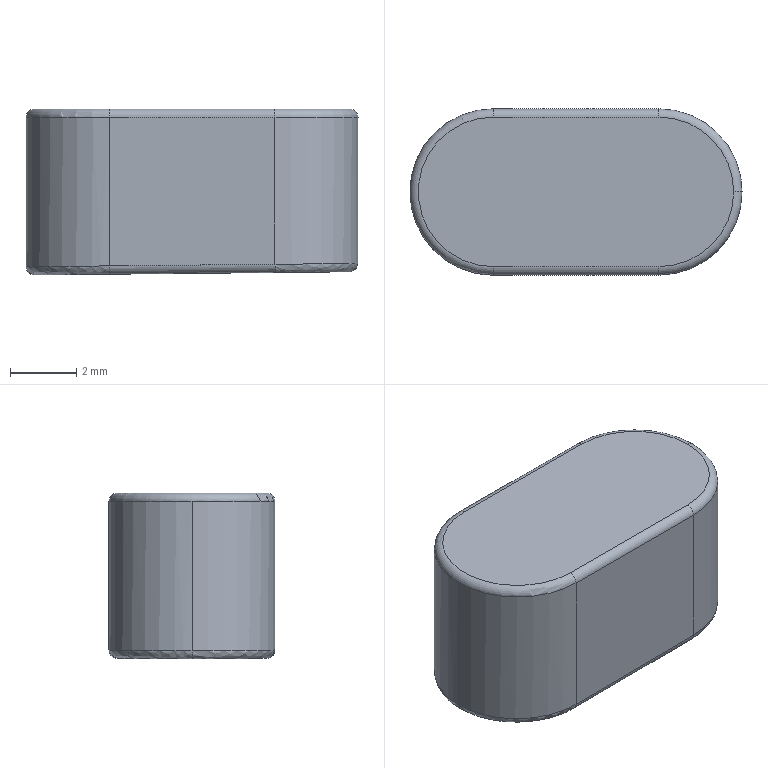Part | SolidWorks | features Cut 1, Extrusion 1, Fillet 1 | 1 solid | 17 faces | box 10 x 5 x 4.997 mm | volume 220.26 mm3 | cylinder 7 | plane 4 | spline 3 | torus 3 | commonest cylinder face diameters 0.5 x4 5 x3
STEP:
#1=CARTESIAN_POINT('',(-4.748,0.,0.002525));
#2=VERTEX_POINT('',#1);
#3=CARTESIAN_POINT('',(-2.498,2.25,0.02502));
#4=VERTEX_POINT('',#3);
#5=CARTESIAN_POINT('',(-4.748,0.,0.002525));
#6=CARTESIAN_POINT('',(-4.748,1.318,0.002525));
#7=CARTESIAN_POINT('',(-3.816,2.25,0.01184));
#8=CARTESIAN_POINT('',(-2.498,2.25,0.02502));
#9=(BOUNDED_CURVE()B_SPLINE_CURVE(3,(#5,#6,#7,#8),.UNSPECIFIED.,.F.,.F.)B_SPLINE_CURVE_WITH_KNOTS((4,4),(0.,1.571),.UNSPECIFIED.)CURVE()GEOMETRIC_REPRESENTATION_ITEM()RATIONAL_B_SPLINE_CURVE((1.,0.8047,0.8047,1.))REPRESENTATION_ITEM(''));
#10=EDGE_CURVE('',#2,#4,#9,.T.);
#11=ORIENTED_EDGE('',*,*,#10,.F.);
#12=CARTESIAN_POINT('',(-5.,0.,0.2525));
#13=VERTEX_POINT('',#12);
#14=CARTESIAN_POINT('',(-4.75,0.,0.2525));
#15=DIRECTION('',(0.,1.,0.));
#16=DIRECTION('',(0.,0.,1.));
#17=AXIS2_PLACEMENT_3D('',#14,#15,#16);
#18=CIRCLE('',#17,0.25);
#19=EDGE_CURVE('',#2,#13,#18,.T.);
#20=ORIENTED_EDGE('',*,*,#19,.T.);
#21=CARTESIAN_POINT('',(-2.5,2.5,0.275));
#22=VERTEX_POINT('',#21);
#23=CARTESIAN_POINT('',(-2.5,2.5,0.275));
#24=CARTESIAN_POINT('',(-3.964,2.5,0.2618));
#25=CARTESIAN_POINT('',(-5.,1.464,0.2525));
#26=CARTESIAN_POINT('',(-5.,0.,0.2525));
#27=(BOUNDED_CURVE()B_SPLINE_CURVE(3,(#23,#24,#25,#26),.UNSPECIFIED.,.F.,.F.)B_SPLINE_CURVE_WITH_KNOTS((4,4),(4.712,6.283),.UNSPECIFIED.)CURVE()GEOMETRIC_REPRESENTATION_ITEM()RATIONAL_B_SPLINE_CURVE((1.,0.8047,0.8047,1.))REPRESENTATION_ITEM(''));
#28=EDGE_CURVE('',#22,#13,#27,.T.);
#29=ORIENTED_EDGE('',*,*,#28,.F.);
#30=CARTESIAN_POINT('',(-2.5,2.25,0.275));
#31=DIRECTION('',(-1.,0.,-0.01));
#32=DIRECTION('',(-0.01,0.,1.));
#33=AXIS2_PLACEMENT_3D('',#30,#31,#32);
#34=CIRCLE('',#33,0.25);
#35=EDGE_CURVE('',#22,#4,#34,.T.);
#36=ORIENTED_EDGE('',*,*,#35,.T.);
#37=EDGE_LOOP('',(#11,#20,#29,#36));
#38=FACE_OUTER_BOUND('',#37,.T.);
#39=CARTESIAN_POINT('',(-2.498,2.25,0.02502));
#40=CARTESIAN_POINT('',(-2.498,2.5,0.02502));
#41=CARTESIAN_POINT('',(-2.5,2.5,0.275));
#42=CARTESIAN_POINT('',(-2.792,2.25,0.02208));
#43=CARTESIAN_POINT('',(-2.825,2.5,0.02175));
#44=CARTESIAN_POINT('',(-2.827,2.5,0.2721));
#45=CARTESIAN_POINT('',(-3.086,2.191,0.01914));
#46=CARTESIAN_POINT('',(-3.152,2.436,0.01848));
#47=CARTESIAN_POINT('',(-3.154,2.435,0.2691));
#48=CARTESIAN_POINT('',(-3.631,1.966,0.01369));
#49=CARTESIAN_POINT('',(-3.757,2.186,0.01243));
#50=CARTESIAN_POINT('',(-3.759,2.184,0.2637));
#51=CARTESIAN_POINT('',(-3.88,1.799,0.0112));
#52=CARTESIAN_POINT('',(-4.035,2.,0.009651));
#53=CARTESIAN_POINT('',(-4.036,1.999,0.2612));
#54=CARTESIAN_POINT('',(-4.297,1.383,0.007032));
#55=CARTESIAN_POINT('',(-4.498,1.538,0.005017));
#56=CARTESIAN_POINT('',(-4.499,1.536,0.257));
#57=CARTESIAN_POINT('',(-4.464,1.133,0.005365));
#58=CARTESIAN_POINT('',(-4.684,1.26,0.003161));
#59=CARTESIAN_POINT('',(-4.684,1.259,0.2554));
#60=CARTESIAN_POINT('',(-4.689,0.5889,0.003111));
#61=CARTESIAN_POINT('',(-4.935,0.655,0.0006517));
#62=CARTESIAN_POINT('',(-4.935,0.6544,0.2531));
#63=CARTESIAN_POINT('',(-4.748,0.2946,0.002525));
#64=CARTESIAN_POINT('',(-5.,0.3276,0.));
#65=CARTESIAN_POINT('',(-5.,0.3273,0.2525));
#66=CARTESIAN_POINT('',(-4.748,0.,0.002525));
#67=CARTESIAN_POINT('',(-5.,0.,0.));
#68=CARTESIAN_POINT('',(-5.,0.,0.2525));
#69=(BOUNDED_SURFACE()B_SPLINE_SURFACE(3,2,((#39,#40,#41),(#42,#43,#44),(#45,#46,#47),(#48,#49,#50),(#51,#52,#53),(#54,#55,#56),(#57,#58,#59),(#60,#61,#62),(#63,#64,#65),(#66,#67,#68)),.UNSPECIFIED.,.F.,.F.,.F.)B_SPLINE_SURFACE_WITH_KNOTS((4,2,2,2,4),(3,3),(4.712,5.105,5.498,5.89,6.283),(0.,1.),.UNSPECIFIED.)GEOMETRIC_REPRESENTATION_ITEM()RATIONAL_B_SPLINE_SURFACE(((1.,0.7071,1.),(1.,0.7066,1.),(1.,0.7062,1.),(1.,0.7053,1.),(1.,0.7049,1.),(1.,0.7043,1.),(1.,0.704,1.),(1.,0.7037,1.),(1.,0.7036,1.),(1.,0.7036,1.)))REPRESENTATION_ITEM('')SURFACE());
#70=ADVANCED_FACE('',(#38),#69,.T.);
#71=CARTESIAN_POINT('',(5.,0.,4.75));
#72=VERTEX_POINT('',#71);
#73=CARTESIAN_POINT('',(2.5,-2.5,4.75));
#74=VERTEX_POINT('',#73);
#75=CARTESIAN_POINT('',(2.5,0.,4.75));
#76=DIRECTION('',(0.,0.,-1.));
#77=DIRECTION('',(1.,0.,0.));
#78=AXIS2_PLACEMENT_3D('',#75,#76,#77);
#79=CIRCLE('',#78,2.5);
#80=EDGE_CURVE('',#72,#74,#79,.T.);
#81=ORIENTED_EDGE('',*,*,#80,.F.);
#82=CARTESIAN_POINT('',(4.75,0.,5.));
#83=VERTEX_POINT('',#82);
#84=CARTESIAN_POINT('',(4.75,0.,4.75));
#85=DIRECTION('',(0.,-1.,0.));
#86=DIRECTION('',(0.,0.,-1.));
#87=AXIS2_PLACEMENT_3D('',#84,#85,#86);
#88=CIRCLE('',#87,0.25);
#89=EDGE_CURVE('',#72,#83,#88,.T.);
#90=ORIENTED_EDGE('',*,*,#89,.T.);
#91=CARTESIAN_POINT('',(2.5,-2.25,5.));
#92=VERTEX_POINT('',#91);
#93=CARTESIAN_POINT('',(2.5,0.,5.));
#94=DIRECTION('',(0.,0.,1.));
#95=DIRECTION('',(1.,0.,0.));
#96=AXIS2_PLACEMENT_3D('',#93,#94,#95);
#97=CIRCLE('',#96,2.25);
#98=EDGE_CURVE('',#92,#83,#97,.T.);
#99=ORIENTED_EDGE('',*,*,#98,.F.);
#100=CARTESIAN_POINT('',(2.5,-2.25,4.75));
#101=DIRECTION('',(-1.,0.,0.));
#102=DIRECTION('',(0.,0.,1.));
#103=AXIS2_PLACEMENT_3D('',#100,#101,#102);
#104=CIRCLE('',#103,0.25);
#105=EDGE_CURVE('',#74,#92,#104,.T.);
#106=ORIENTED_EDGE('',*,*,#105,.F.);
#107=EDGE_LOOP('',(#81,#90,#99,#106));
#108=FACE_OUTER_BOUND('',#107,.T.);
#109=CARTESIAN_POINT('',(2.5,0.,4.75));
#110=DIRECTION('',(0.,0.,1.));
#111=DIRECTION('',(1.,0.,0.));
#112=AXIS2_PLACEMENT_3D('',#109,#110,#111);
#113=TOROIDAL_SURFACE('',#112,2.25,0.25);
#114=ADVANCED_FACE('',(#108),#113,.T.);
#115=CARTESIAN_POINT('',(-2.5,-2.5,4.75));
#116=VERTEX_POINT('',#115);
#117=CARTESIAN_POINT('',(-5.,0.,4.75));
#118=VERTEX_POINT('',#117);
#119=CARTESIAN_POINT('',(-2.5,0.,4.75));
#120=DIRECTION('',(0.,0.,-1.));
#121=DIRECTION('',(1.,0.,0.));
#122=AXIS2_PLACEMENT_3D('',#119,#120,#121);
#123=CIRCLE('',#122,2.5);
#124=EDGE_CURVE('',#116,#118,#123,.T.);
#125=ORIENTED_EDGE('',*,*,#124,.T.);
#126=CARTESIAN_POINT('',(-5.,0.,5.));
#127=DIRECTION('',(0.,0.,-1.));
#128=VECTOR('',#127,1000.);
#129=LINE('',#126,#128);
#130=EDGE_CURVE('',#118,#13,#129,.T.);
#131=ORIENTED_EDGE('',*,*,#130,.T.);
#132=CARTESIAN_POINT('',(-2.5,-2.5,0.275));
#133=VERTEX_POINT('',#132);
#134=CARTESIAN_POINT('',(-5.,0.,0.2525));
#135=CARTESIAN_POINT('',(-5.,-1.464,0.2525));
#136=CARTESIAN_POINT('',(-3.964,-2.5,0.2618));
#137=CARTESIAN_POINT('',(-2.5,-2.5,0.275));
#138=(BOUNDED_CURVE()B_SPLINE_CURVE(3,(#134,#135,#136,#137),.UNSPECIFIED.,.F.,.F.)B_SPLINE_CURVE_WITH_KNOTS((4,4),(0.,1.571),.UNSPECIFIED.)CURVE()GEOMETRIC_REPRESENTATION_ITEM()RATIONAL_B_SPLINE_CURVE((1.,0.8047,0.8047,1.))REPRESENTATION_ITEM(''));
#139=EDGE_CURVE('',#13,#133,#138,.T.);
#140=ORIENTED_EDGE('',*,*,#139,.T.);
#141=CARTESIAN_POINT('',(-2.5,-2.5,5.));
#142=DIRECTION('',(0.,0.,-1.));
#143=VECTOR('',#142,1000.);
#144=LINE('',#141,#143);
#145=EDGE_CURVE('',#116,#133,#144,.T.);
#146=ORIENTED_EDGE('',*,*,#145,.F.);
#147=EDGE_LOOP('',(#125,#131,#140,#146));
#148=FACE_OUTER_BOUND('',#147,.T.);
#149=CARTESIAN_POINT('',(-2.5,0.,5.));
#150=DIRECTION('',(0.,0.,-1.));
#151=DIRECTION('',(-1.,0.,0.));
#152=AXIS2_PLACEMENT_3D('',#149,#150,#151);
#153=CYLINDRICAL_SURFACE('',#152,2.5);
#154=ADVANCED_FACE('',(#148),#153,.T.);
#155=ORIENTED_EDGE('',*,*,#130,.F.);
#156=CARTESIAN_POINT('',(-2.5,2.5,4.75));
#157=VERTEX_POINT('',#156);
#158=CARTESIAN_POINT('',(-2.5,0.,4.75));
#159=DIRECTION('',(0.,0.,-1.));
#160=DIRECTION('',(1.,0.,0.));
#161=AXIS2_PLACEMENT_3D('',#158,#159,#160);
#162=CIRCLE('',#161,2.5);
#163=EDGE_CURVE('',#118,#157,#162,.T.);
#164=ORIENTED_EDGE('',*,*,#163,.T.);
#165=CARTESIAN_POINT('',(-2.5,2.5,5.));
#166=DIRECTION('',(0.,0.,-1.));
#167=VECTOR('',#166,1000.);
#168=LINE('',#165,#167);
#169=EDGE_CURVE('',#157,#22,#168,.T.);
#170=ORIENTED_EDGE('',*,*,#169,.T.);
#171=ORIENTED_EDGE('',*,*,#28,.T.);
#172=EDGE_LOOP('',(#155,#164,#170,#171));
#173=FACE_OUTER_BOUND('',#172,.T.);
#174=CARTESIAN_POINT('',(-2.5,0.,5.));
#175=DIRECTION('',(0.,0.,-1.));
#176=DIRECTION('',(-1.,0.,0.));
#177=AXIS2_PLACEMENT_3D('',#174,#175,#176);
#178=CYLINDRICAL_SURFACE('',#177,2.5);
#179=ADVANCED_FACE('',(#173),#178,.T.);
#180=CARTESIAN_POINT('',(2.5,-2.5,0.325));
#181=VERTEX_POINT('',#180);
#182=CARTESIAN_POINT('',(2.5,-2.5,5.));
#183=DIRECTION('',(0.,0.,-1.));
#184=VECTOR('',#183,1000.);
#185=LINE('',#182,#184);
#186=EDGE_CURVE('',#74,#181,#185,.T.);
#187=ORIENTED_EDGE('',*,*,#186,.F.);
#188=CARTESIAN_POINT('',(-2.5,-2.5,4.75));
#189=DIRECTION('',(-1.,0.,0.));
#190=VECTOR('',#189,1000.);
#191=LINE('',#188,#190);
#192=EDGE_CURVE('',#74,#116,#191,.T.);
#193=ORIENTED_EDGE('',*,*,#192,.T.);
#194=ORIENTED_EDGE('',*,*,#145,.T.);
#195=CARTESIAN_POINT('',(2.547,-2.5,0.3255));
#196=DIRECTION('',(1.,0.,0.01));
#197=VECTOR('',#196,1000.);
#198=LINE('',#195,#197);
#199=EDGE_CURVE('',#133,#181,#198,.T.);
#200=ORIENTED_EDGE('',*,*,#199,.T.);
#201=EDGE_LOOP('',(#187,#193,#194,#200));
#202=FACE_OUTER_BOUND('',#201,.T.);
#203=CARTESIAN_POINT('',(2.5,-2.5,5.));
#204=DIRECTION('',(0.,1.,0.));
#205=DIRECTION('',(0.,0.,1.));
#206=AXIS2_PLACEMENT_3D('',#203,#204,#205);
#207=PLANE('',#206);
#208=ADVANCED_FACE('',(#202),#207,.F.);
#209=ORIENTED_EDGE('',*,*,#186,.T.);
#210=CARTESIAN_POINT('',(2.5,2.5,0.325));
#211=VERTEX_POINT('',#210);
#212=CARTESIAN_POINT('',(2.5,-2.5,0.325));
#213=CARTESIAN_POINT('',(7.5,-2.5,0.37));
#214=CARTESIAN_POINT('',(7.5,2.5,0.37));
#215=CARTESIAN_POINT('',(2.5,2.5,0.325));
#216=(BOUNDED_CURVE()B_SPLINE_CURVE(3,(#212,#213,#214,#215),.UNSPECIFIED.,.F.,.T.)B_SPLINE_CURVE_WITH_KNOTS((4,4),(1.571,4.712),.UNSPECIFIED.)CURVE()GEOMETRIC_REPRESENTATION_ITEM()RATIONAL_B_SPLINE_CURVE((1.,0.3333,0.3333,1.))REPRESENTATION_ITEM(''));
#217=EDGE_CURVE('',#181,#211,#216,.T.);
#218=ORIENTED_EDGE('',*,*,#217,.T.);
#219=CARTESIAN_POINT('',(2.5,2.5,4.75));
#220=VERTEX_POINT('',#219);
#221=CARTESIAN_POINT('',(2.5,2.5,5.));
#222=DIRECTION('',(0.,0.,-1.));
#223=VECTOR('',#222,1000.);
#224=LINE('',#221,#223);
#225=EDGE_CURVE('',#220,#211,#224,.T.);
#226=ORIENTED_EDGE('',*,*,#225,.F.);
#227=CARTESIAN_POINT('',(2.5,0.,4.75));
#228=DIRECTION('',(0.,0.,-1.));
#229=DIRECTION('',(1.,0.,0.));
#230=AXIS2_PLACEMENT_3D('',#227,#228,#229);
#231=CIRCLE('',#230,2.5);
#232=EDGE_CURVE('',#220,#72,#231,.T.);
#233=ORIENTED_EDGE('',*,*,#232,.T.);
#234=ORIENTED_EDGE('',*,*,#80,.T.);
#235=EDGE_LOOP('',(#209,#218,#226,#233,#234));
#236=FACE_OUTER_BOUND('',#235,.T.);
#237=CARTESIAN_POINT('',(2.5,0.,5.));
#238=DIRECTION('',(0.,0.,-1.));
#239=DIRECTION('',(-1.,0.,0.));
#240=AXIS2_PLACEMENT_3D('',#237,#238,#239);
#241=CYLINDRICAL_SURFACE('',#240,2.5);
#242=ADVANCED_FACE('',(#236),#241,.T.);
#243=ORIENTED_EDGE('',*,*,#169,.F.);
#244=CARTESIAN_POINT('',(2.5,2.5,4.75));
#245=DIRECTION('',(1.,0.,0.));
#246=VECTOR('',#245,1000.);
#247=LINE('',#244,#246);
#248=EDGE_CURVE('',#157,#220,#247,.T.);
#249=ORIENTED_EDGE('',*,*,#248,.T.);
#250=ORIENTED_EDGE('',*,*,#225,.T.);
#251=CARTESIAN_POINT('',(-2.453,2.5,0.2755));
#252=DIRECTION('',(-1.,0.,-0.01));
#253=VECTOR('',#252,1000.);
#254=LINE('',#251,#253);
#255=EDGE_CURVE('',#211,#22,#254,.T.);
#256=ORIENTED_EDGE('',*,*,#255,.T.);
#257=EDGE_LOOP('',(#243,#249,#250,#256));
#258=FACE_OUTER_BOUND('',#257,.T.);
#259=CARTESIAN_POINT('',(-2.5,2.5,5.));
#260=DIRECTION('',(0.,-1.,0.));
#261=DIRECTION('',(0.,0.,-1.));
#262=AXIS2_PLACEMENT_3D('',#259,#260,#261);
#263=PLANE('',#262);
#264=ADVANCED_FACE('',(#258),#263,.F.);
#265=CARTESIAN_POINT('',(-2.5,2.25,5.));
#266=VERTEX_POINT('',#265);
#267=CARTESIAN_POINT('',(-2.5,-2.25,5.));
#268=VERTEX_POINT('',#267);
#269=CARTESIAN_POINT('',(-2.5,0.,5.));
#270=DIRECTION('',(0.,0.,1.));
#271=DIRECTION('',(1.,0.,0.));
#272=AXIS2_PLACEMENT_3D('',#269,#270,#271);
#273=CIRCLE('',#272,2.25);
#274=EDGE_CURVE('',#266,#268,#273,.T.);
#275=ORIENTED_EDGE('',*,*,#274,.T.);
#276=CARTESIAN_POINT('',(2.5,-2.25,5.));
#277=DIRECTION('',(1.,0.,0.));
#278=VECTOR('',#277,1000.);
#279=LINE('',#276,#278);
#280=EDGE_CURVE('',#268,#92,#279,.T.);
#281=ORIENTED_EDGE('',*,*,#280,.T.);
#282=ORIENTED_EDGE('',*,*,#98,.T.);
#283=CARTESIAN_POINT('',(2.5,2.25,5.));
#284=VERTEX_POINT('',#283);
#285=CARTESIAN_POINT('',(2.5,0.,5.));
#286=DIRECTION('',(0.,0.,1.));
#287=DIRECTION('',(1.,0.,0.));
#288=AXIS2_PLACEMENT_3D('',#285,#286,#287);
#289=CIRCLE('',#288,2.25);
#290=EDGE_CURVE('',#83,#284,#289,.T.);
#291=ORIENTED_EDGE('',*,*,#290,.T.);
#292=CARTESIAN_POINT('',(-2.5,2.25,5.));
#293=DIRECTION('',(-1.,0.,0.));
#294=VECTOR('',#293,1000.);
#295=LINE('',#292,#294);
#296=EDGE_CURVE('',#284,#266,#295,.T.);
#297=ORIENTED_EDGE('',*,*,#296,.T.);
#298=EDGE_LOOP('',(#275,#281,#282,#291,#297));
#299=FACE_OUTER_BOUND('',#298,.T.);
#300=CARTESIAN_POINT('',(-2.5,0.,5.));
#301=DIRECTION('',(0.,0.,1.));
#302=DIRECTION('',(1.,0.,0.));
#303=AXIS2_PLACEMENT_3D('',#300,#301,#302);
#304=PLANE('',#303);
#305=ADVANCED_FACE('',(#299),#304,.T.);
#306=CARTESIAN_POINT('',(2.502,-2.25,0.07502));
#307=VERTEX_POINT('',#306);
#308=CARTESIAN_POINT('',(-2.498,-2.25,0.02502));
#309=VERTEX_POINT('',#308);
#310=CARTESIAN_POINT('',(-5.,-2.25,0.));
#311=DIRECTION('',(-1.,0.,-0.01));
#312=VECTOR('',#311,1000.);
#313=LINE('',#310,#312);
#314=EDGE_CURVE('',#307,#309,#313,.T.);
#315=ORIENTED_EDGE('',*,*,#314,.T.);
#316=CARTESIAN_POINT('',(-2.498,-2.25,0.02502));
#317=CARTESIAN_POINT('',(-3.816,-2.25,0.01184));
#318=CARTESIAN_POINT('',(-4.748,-1.318,0.002525));
#319=CARTESIAN_POINT('',(-4.748,0.,0.002525));
#320=(BOUNDED_CURVE()B_SPLINE_CURVE(3,(#316,#317,#318,#319),.UNSPECIFIED.,.F.,.F.)B_SPLINE_CURVE_WITH_KNOTS((4,4),(4.712,6.283),.UNSPECIFIED.)CURVE()GEOMETRIC_REPRESENTATION_ITEM()RATIONAL_B_SPLINE_CURVE((1.,0.8047,0.8047,1.))REPRESENTATION_ITEM(''));
#321=EDGE_CURVE('',#309,#2,#320,.T.);
#322=ORIENTED_EDGE('',*,*,#321,.T.);
#323=ORIENTED_EDGE('',*,*,#10,.T.);
#324=CARTESIAN_POINT('',(2.502,2.25,0.07502));
#325=VERTEX_POINT('',#324);
#326=CARTESIAN_POINT('',(-5.,2.25,0.));
#327=DIRECTION('',(1.,0.,0.01));
#328=VECTOR('',#327,1000.);
#329=LINE('',#326,#328);
#330=EDGE_CURVE('',#4,#325,#329,.T.);
#331=ORIENTED_EDGE('',*,*,#330,.T.);
#332=CARTESIAN_POINT('',(2.502,2.25,0.07502));
#333=CARTESIAN_POINT('',(7.002,2.25,0.12));
#334=CARTESIAN_POINT('',(7.002,-2.25,0.12));
#335=CARTESIAN_POINT('',(2.502,-2.25,0.07502));
#336=(BOUNDED_CURVE()B_SPLINE_CURVE(3,(#332,#333,#334,#335),.UNSPECIFIED.,.F.,.F.)B_SPLINE_CURVE_WITH_KNOTS((4,4),(1.571,4.712),.UNSPECIFIED.)CURVE()GEOMETRIC_REPRESENTATION_ITEM()RATIONAL_B_SPLINE_CURVE((1.,0.3333,0.3333,1.))REPRESENTATION_ITEM(''));
#337=EDGE_CURVE('',#325,#307,#336,.T.);
#338=ORIENTED_EDGE('',*,*,#337,.T.);
#339=EDGE_LOOP('',(#315,#322,#323,#331,#338));
#340=FACE_OUTER_BOUND('',#339,.T.);
#341=CARTESIAN_POINT('',(-5.,-2.5,0.));
#342=DIRECTION('',(-0.01,0.,1.));
#343=DIRECTION('',(1.,0.,0.01));
#344=AXIS2_PLACEMENT_3D('',#341,#342,#343);
#345=PLANE('',#344);
#346=ADVANCED_FACE('',(#340),#345,.F.);
#347=CARTESIAN_POINT('',(2.5,2.25,4.75));
#348=DIRECTION('',(1.,0.,0.));
#349=DIRECTION('',(0.,0.,-1.));
#350=AXIS2_PLACEMENT_3D('',#347,#348,#349);
#351=CIRCLE('',#350,0.25);
#352=EDGE_CURVE('',#220,#284,#351,.T.);
#353=ORIENTED_EDGE('',*,*,#352,.F.);
#354=ORIENTED_EDGE('',*,*,#248,.F.);
#355=CARTESIAN_POINT('',(-2.5,2.25,4.75));
#356=DIRECTION('',(-1.,0.,0.));
#357=DIRECTION('',(0.,0.,1.));
#358=AXIS2_PLACEMENT_3D('',#355,#356,#357);
#359=CIRCLE('',#358,0.25);
#360=EDGE_CURVE('',#266,#157,#359,.T.);
#361=ORIENTED_EDGE('',*,*,#360,.F.);
#362=ORIENTED_EDGE('',*,*,#296,.F.);
#363=EDGE_LOOP('',(#353,#354,#361,#362));
#364=FACE_OUTER_BOUND('',#363,.T.);
#365=CARTESIAN_POINT('',(-2.5,2.25,4.75));
#366=DIRECTION('',(1.,0.,0.));
#367=DIRECTION('',(0.,0.,-1.));
#368=AXIS2_PLACEMENT_3D('',#365,#366,#367);
#369=CYLINDRICAL_SURFACE('',#368,0.25);
#370=ADVANCED_FACE('',(#364),#369,.T.);
#371=ORIENTED_EDGE('',*,*,#360,.T.);
#372=ORIENTED_EDGE('',*,*,#163,.F.);
#373=ORIENTED_EDGE('',*,*,#124,.F.);
#374=CARTESIAN_POINT('',(-2.5,-2.25,4.75));
#375=DIRECTION('',(1.,0.,0.));
#376=DIRECTION('',(0.,0.,-1.));
#377=AXIS2_PLACEMENT_3D('',#374,#375,#376);
#378=CIRCLE('',#377,0.25);
#379=EDGE_CURVE('',#268,#116,#378,.T.);
#380=ORIENTED_EDGE('',*,*,#379,.F.);
#381=ORIENTED_EDGE('',*,*,#274,.F.);
#382=EDGE_LOOP('',(#371,#372,#373,#380,#381));
#383=FACE_OUTER_BOUND('',#382,.T.);
#384=CARTESIAN_POINT('',(-2.5,0.,4.75));
#385=DIRECTION('',(0.,0.,1.));
#386=DIRECTION('',(1.,0.,0.));
#387=AXIS2_PLACEMENT_3D('',#384,#385,#386);
#388=TOROIDAL_SURFACE('',#387,2.25,0.25);
#389=ADVANCED_FACE('',(#383),#388,.T.);
#390=ORIENTED_EDGE('',*,*,#89,.F.);
#391=ORIENTED_EDGE('',*,*,#232,.F.);
#392=ORIENTED_EDGE('',*,*,#352,.T.);
#393=ORIENTED_EDGE('',*,*,#290,.F.);
#394=EDGE_LOOP('',(#390,#391,#392,#393));
#395=FACE_OUTER_BOUND('',#394,.T.);
#396=CARTESIAN_POINT('',(2.5,0.,4.75));
#397=DIRECTION('',(0.,0.,1.));
#398=DIRECTION('',(1.,0.,0.));
#399=AXIS2_PLACEMENT_3D('',#396,#397,#398);
#400=TOROIDAL_SURFACE('',#399,2.25,0.25);
#401=ADVANCED_FACE('',(#395),#400,.T.);
#402=ORIENTED_EDGE('',*,*,#379,.T.);
#403=ORIENTED_EDGE('',*,*,#192,.F.);
#404=ORIENTED_EDGE('',*,*,#105,.T.);
#405=ORIENTED_EDGE('',*,*,#280,.F.);
#406=EDGE_LOOP('',(#402,#403,#404,#405));
#407=FACE_OUTER_BOUND('',#406,.T.);
#408=CARTESIAN_POINT('',(-2.5,-2.25,4.75));
#409=DIRECTION('',(-1.,0.,0.));
#410=DIRECTION('',(0.,0.,1.));
#411=AXIS2_PLACEMENT_3D('',#408,#409,#410);
#412=CYLINDRICAL_SURFACE('',#411,0.25);
#413=ADVANCED_FACE('',(#407),#412,.T.);
#414=CARTESIAN_POINT('',(2.5,-2.25,0.325));
#415=DIRECTION('',(-1.,0.,-0.01));
#416=DIRECTION('',(-0.01,0.,1.));
#417=AXIS2_PLACEMENT_3D('',#414,#415,#416);
#418=CIRCLE('',#417,0.25);
#419=EDGE_CURVE('',#307,#181,#418,.T.);
#420=ORIENTED_EDGE('',*,*,#419,.F.);
#421=ORIENTED_EDGE('',*,*,#337,.F.);
#422=CARTESIAN_POINT('',(2.5,2.25,0.325));
#423=DIRECTION('',(-1.,0.,-0.01));
#424=DIRECTION('',(-0.01,0.,1.));
#425=AXIS2_PLACEMENT_3D('',#422,#423,#424);
#426=CIRCLE('',#425,0.25);
#427=EDGE_CURVE('',#211,#325,#426,.T.);
#428=ORIENTED_EDGE('',*,*,#427,.F.);
#429=ORIENTED_EDGE('',*,*,#217,.F.);
#430=EDGE_LOOP('',(#420,#421,#428,#429));
#431=FACE_OUTER_BOUND('',#430,.T.);
#432=CARTESIAN_POINT('',(2.502,-2.25,0.07502));
#433=CARTESIAN_POINT('',(2.502,-2.5,0.07502));
#434=CARTESIAN_POINT('',(2.5,-2.5,0.325));
#435=CARTESIAN_POINT('',(2.797,-2.25,0.07797));
#436=CARTESIAN_POINT('',(2.83,-2.5,0.0783));
#437=CARTESIAN_POINT('',(2.827,-2.5,0.328));
#438=CARTESIAN_POINT('',(3.091,-2.191,0.08091));
#439=CARTESIAN_POINT('',(3.157,-2.434,0.08157));
#440=CARTESIAN_POINT('',(3.154,-2.435,0.3309));
#441=CARTESIAN_POINT('',(3.636,-1.966,0.08636));
#442=CARTESIAN_POINT('',(3.761,-2.183,0.08761));
#443=CARTESIAN_POINT('',(3.759,-2.184,0.3363));
#444=CARTESIAN_POINT('',(3.885,-1.799,0.08885));
#445=CARTESIAN_POINT('',(4.038,-1.998,0.09038));
#446=CARTESIAN_POINT('',(4.036,-1.999,0.3388));
#447=CARTESIAN_POINT('',(4.302,-1.383,0.09302));
#448=CARTESIAN_POINT('',(4.5,-1.535,0.095));
#449=CARTESIAN_POINT('',(4.499,-1.536,0.343));
#450=CARTESIAN_POINT('',(4.469,-1.133,0.09469));
#451=CARTESIAN_POINT('',(4.685,-1.258,0.09685));
#452=CARTESIAN_POINT('',(4.684,-1.259,0.3447));
#453=CARTESIAN_POINT('',(4.694,-0.5889,0.09694));
#454=CARTESIAN_POINT('',(4.935,-0.6538,0.09935));
#455=CARTESIAN_POINT('',(4.935,-0.6544,0.3469));
#456=CARTESIAN_POINT('',(4.752,-0.2945,0.09752));
#457=CARTESIAN_POINT('',(5.,-0.3269,0.1));
#458=CARTESIAN_POINT('',(5.,-0.3272,0.3475));
#459=CARTESIAN_POINT('',(4.752,0.2945,0.09752));
#460=CARTESIAN_POINT('',(5.,0.3269,0.1));
#461=CARTESIAN_POINT('',(5.,0.3272,0.3475));
#462=CARTESIAN_POINT('',(4.694,0.5889,0.09694));
#463=CARTESIAN_POINT('',(4.935,0.6538,0.09935));
#464=CARTESIAN_POINT('',(4.935,0.6544,0.3469));
#465=CARTESIAN_POINT('',(4.469,1.133,0.09469));
#466=CARTESIAN_POINT('',(4.685,1.258,0.09685));
#467=CARTESIAN_POINT('',(4.684,1.259,0.3447));
#468=CARTESIAN_POINT('',(4.302,1.383,0.09302));
#469=CARTESIAN_POINT('',(4.5,1.535,0.095));
#470=CARTESIAN_POINT('',(4.499,1.536,0.343));
#471=CARTESIAN_POINT('',(3.885,1.799,0.08885));
#472=CARTESIAN_POINT('',(4.038,1.998,0.09038));
#473=CARTESIAN_POINT('',(4.036,1.999,0.3388));
#474=CARTESIAN_POINT('',(3.636,1.966,0.08636));
#475=CARTESIAN_POINT('',(3.761,2.183,0.08761));
#476=CARTESIAN_POINT('',(3.759,2.184,0.3363));
#477=CARTESIAN_POINT('',(3.091,2.191,0.08091));
#478=CARTESIAN_POINT('',(3.157,2.434,0.08157));
#479=CARTESIAN_POINT('',(3.154,2.435,0.3309));
#480=CARTESIAN_POINT('',(2.797,2.25,0.07797));
#481=CARTESIAN_POINT('',(2.83,2.5,0.0783));
#482=CARTESIAN_POINT('',(2.827,2.5,0.328));
#483=CARTESIAN_POINT('',(2.502,2.25,0.07502));
#484=CARTESIAN_POINT('',(2.502,2.5,0.07502));
#485=CARTESIAN_POINT('',(2.5,2.5,0.325));
#486=(BOUNDED_SURFACE()B_SPLINE_SURFACE(3,2,((#432,#433,#434),(#435,#436,#437),(#438,#439,#440),(#441,#442,#443),(#444,#445,#446),(#447,#448,#449),(#450,#451,#452),(#453,#454,#455),(#456,#457,#458),(#459,#460,#461),(#462,#463,#464),(#465,#466,#467),(#468,#469,#470),(#471,#472,#473),(#474,#475,#476),(#477,#478,#479),(#480,#481,#482),(#483,#484,#485)),.UNSPECIFIED.,.F.,.F.,.F.)B_SPLINE_SURFACE_WITH_KNOTS((4,2,2,2,2,2,2,2,4),(3,3),(1.571,1.963,2.356,2.749,3.142,3.534,3.927,4.32,4.712),(0.,1.),.UNSPECIFIED.)GEOMETRIC_REPRESENTATION_ITEM()RATIONAL_B_SPLINE_SURFACE(((1.,0.7071,1.),(1.,0.7076,1.),(1.,0.708,1.),(1.,0.7089,1.),(1.,0.7093,1.),(1.,0.7099,1.),(1.,0.7102,1.),(1.,0.7105,1.),(1.,0.7106,1.),(1.,0.7106,1.),(1.,0.7105,1.),(1.,0.7102,1.),(1.,0.7099,1.),(1.,0.7093,1.),(1.,0.7089,1.),(1.,0.708,1.),(1.,0.7076,1.),(1.,0.7071,1.)))REPRESENTATION_ITEM('')SURFACE());
#487=ADVANCED_FACE('',(#431),#486,.T.);
#488=ORIENTED_EDGE('',*,*,#427,.T.);
#489=ORIENTED_EDGE('',*,*,#330,.F.);
#490=ORIENTED_EDGE('',*,*,#35,.F.);
#491=ORIENTED_EDGE('',*,*,#255,.F.);
#492=EDGE_LOOP('',(#488,#489,#490,#491));
#493=FACE_OUTER_BOUND('',#492,.T.);
#494=CARTESIAN_POINT('',(-5.002,2.25,0.25));
#495=DIRECTION('',(1.,0.,0.01));
#496=DIRECTION('',(0.01,0.,-1.));
#497=AXIS2_PLACEMENT_3D('',#494,#495,#496);
#498=CYLINDRICAL_SURFACE('',#497,0.25);
#499=ADVANCED_FACE('',(#493),#498,.T.);
#500=ORIENTED_EDGE('',*,*,#419,.T.);
#501=ORIENTED_EDGE('',*,*,#199,.F.);
#502=CARTESIAN_POINT('',(-2.5,-2.25,0.275));
#503=DIRECTION('',(-1.,0.,-0.01));
#504=DIRECTION('',(-0.01,0.,1.));
#505=AXIS2_PLACEMENT_3D('',#502,#503,#504);
#506=CIRCLE('',#505,0.25);
#507=EDGE_CURVE('',#309,#133,#506,.T.);
#508=ORIENTED_EDGE('',*,*,#507,.F.);
#509=ORIENTED_EDGE('',*,*,#314,.F.);
#510=EDGE_LOOP('',(#500,#501,#508,#509));
#511=FACE_OUTER_BOUND('',#510,.T.);
#512=CARTESIAN_POINT('',(2.547,-2.25,0.3255));
#513=DIRECTION('',(1.,0.,0.01));
#514=DIRECTION('',(0.01,0.,-1.));
#515=AXIS2_PLACEMENT_3D('',#512,#513,#514);
#516=CYLINDRICAL_SURFACE('',#515,0.25);
#517=ADVANCED_FACE('',(#511),#516,.T.);
#518=ORIENTED_EDGE('',*,*,#19,.F.);
#519=ORIENTED_EDGE('',*,*,#321,.F.);
#520=ORIENTED_EDGE('',*,*,#507,.T.);
#521=ORIENTED_EDGE('',*,*,#139,.F.);
#522=EDGE_LOOP('',(#518,#519,#520,#521));
#523=FACE_OUTER_BOUND('',#522,.T.);
#524=CARTESIAN_POINT('',(-4.748,0.,0.002525));
#525=CARTESIAN_POINT('',(-5.,0.,0.));
#526=CARTESIAN_POINT('',(-5.,0.,0.2525));
#527=CARTESIAN_POINT('',(-4.748,-0.2946,0.002525));
#528=CARTESIAN_POINT('',(-5.,-0.3276,0.));
#529=CARTESIAN_POINT('',(-5.,-0.3273,0.2525));
#530=CARTESIAN_POINT('',(-4.689,-0.5889,0.003111));
#531=CARTESIAN_POINT('',(-4.935,-0.655,0.0006517));
#532=CARTESIAN_POINT('',(-4.935,-0.6544,0.2531));
#533=CARTESIAN_POINT('',(-4.464,-1.133,0.005365));
#534=CARTESIAN_POINT('',(-4.684,-1.26,0.003161));
#535=CARTESIAN_POINT('',(-4.684,-1.259,0.2554));
#536=CARTESIAN_POINT('',(-4.297,-1.383,0.007032));
#537=CARTESIAN_POINT('',(-4.498,-1.538,0.005017));
#538=CARTESIAN_POINT('',(-4.499,-1.536,0.257));
#539=CARTESIAN_POINT('',(-3.88,-1.799,0.0112));
#540=CARTESIAN_POINT('',(-4.035,-2.,0.009651));
#541=CARTESIAN_POINT('',(-4.036,-1.999,0.2612));
#542=CARTESIAN_POINT('',(-3.631,-1.966,0.01369));
#543=CARTESIAN_POINT('',(-3.757,-2.186,0.01243));
#544=CARTESIAN_POINT('',(-3.759,-2.184,0.2637));
#545=CARTESIAN_POINT('',(-3.086,-2.191,0.01914));
#546=CARTESIAN_POINT('',(-3.152,-2.436,0.01848));
#547=CARTESIAN_POINT('',(-3.154,-2.435,0.2691));
#548=CARTESIAN_POINT('',(-2.792,-2.25,0.02208));
#549=CARTESIAN_POINT('',(-2.825,-2.5,0.02175));
#550=CARTESIAN_POINT('',(-2.827,-2.5,0.2721));
#551=CARTESIAN_POINT('',(-2.498,-2.25,0.02502));
#552=CARTESIAN_POINT('',(-2.498,-2.5,0.02502));
#553=CARTESIAN_POINT('',(-2.5,-2.5,0.275));
#554=(BOUNDED_SURFACE()B_SPLINE_SURFACE(3,2,((#524,#525,#526),(#527,#528,#529),(#530,#531,#532),(#533,#534,#535),(#536,#537,#538),(#539,#540,#541),(#542,#543,#544),(#545,#546,#547),(#548,#549,#550),(#551,#552,#553)),.UNSPECIFIED.,.F.,.F.,.F.)B_SPLINE_SURFACE_WITH_KNOTS((4,2,2,2,4),(3,3),(0.,0.3927,0.7854,1.178,1.571),(0.,1.),.UNSPECIFIED.)GEOMETRIC_REPRESENTATION_ITEM()RATIONAL_B_SPLINE_SURFACE(((1.,0.7036,1.),(1.,0.7036,1.),(1.,0.7037,1.),(1.,0.704,1.),(1.,0.7043,1.),(1.,0.7049,1.),(1.,0.7053,1.),(1.,0.7062,1.),(1.,0.7066,1.),(1.,0.7071,1.)))REPRESENTATION_ITEM('')SURFACE());
#555=ADVANCED_FACE('',(#523),#554,.T.);
#556=CLOSED_SHELL('',(#70,#114,#154,#179,#208,#242,#264,#305,#346,#370,#389,#401,#413,#487,#499,#517,#555));
#557=MANIFOLD_SOLID_BREP('',#556);
#558=CARTESIAN_POINT('',(0.,0.,0.));
#559=DIRECTION('',(0.,0.,1.));
#560=DIRECTION('',(1.,0.,0.));
#561=AXIS2_PLACEMENT_3D('',#558,#559,#560);
#562=(LENGTH_UNIT()NAMED_UNIT(*)SI_UNIT(.MILLI.,.METRE.));
#563=UNCERTAINTY_MEASURE_WITH_UNIT(LENGTH_MEASURE(0.00001),#562,'','');
#564=(NAMED_UNIT(*)PLANE_ANGLE_UNIT()SI_UNIT($,.RADIAN.));
#565=(NAMED_UNIT(*)SI_UNIT($,.STERADIAN.)SOLID_ANGLE_UNIT());
#566=(GEOMETRIC_REPRESENTATION_CONTEXT(3)GLOBAL_UNCERTAINTY_ASSIGNED_CONTEXT((#563))GLOBAL_UNIT_ASSIGNED_CONTEXT((#562,#564,#565))REPRESENTATION_CONTEXT('',''));
#567=ADVANCED_BREP_SHAPE_REPRESENTATION('',(#557,#561),#566);